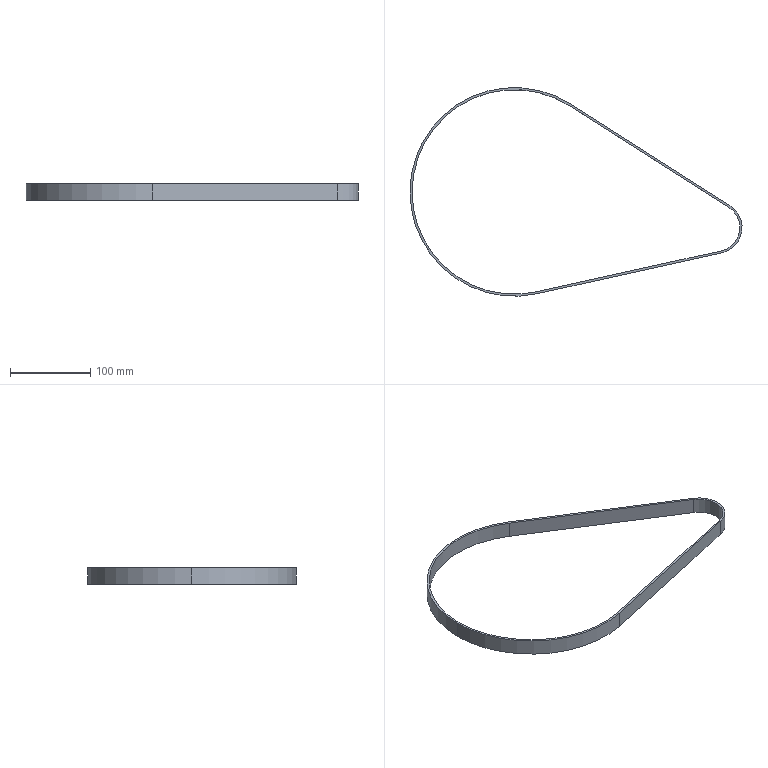Part | STEP file | Belt 1-8^ tube-changer assembly SGN-2 | 1 solid | 12 faces | box 413.576 x 259.89 x 20 mm | volume 55011 mm3 | cylinder 6 | plane 6 | commonest cylinder face diameters 254.65 x2 259.89 x2 59.74 x1 64.98 x1
STEP:
#1=CARTESIAN_POINT('',(0.,0.,0.));
#2=DIRECTION('',(0.,0.,1.));
#3=DIRECTION('',(1.,0.,0.));
#4=AXIS2_PLACEMENT_3D('',#1,#2,#3);
#5=CARTESIAN_POINT('',(-174.515,128.116,20.));
#6=VERTEX_POINT('',#5);
#7=CARTESIAN_POINT('',(-174.515,128.116,0.));
#8=VERTEX_POINT('',#7);
#9=CARTESIAN_POINT('',(-174.515,128.116,20.));
#10=DIRECTION('',(0.,0.,-1.));
#11=VECTOR('',#10,1.);
#12=LINE('',#9,#11);
#13=CARTESIAN_POINT('',(-242.865,20.692,20.));
#14=DIRECTION('',(0.,0.,-1.));
#15=DIRECTION('',(-1.,0.,0.));
#16=AXIS2_PLACEMENT_3D('',#13,#14,#15);
#17=CYLINDRICAL_SURFACE('',#16,127.325);
#18=CARTESIAN_POINT('',(2.137,0.));
#19=DIRECTION('',(0.,1.));
#20=VECTOR('',#19,1.);
#21=LINE('',#18,#20);
#22=(GEOMETRIC_REPRESENTATION_CONTEXT(2)PARAMETRIC_REPRESENTATION_CONTEXT()REPRESENTATION_CONTEXT('',''));
#23=DEFINITIONAL_REPRESENTATION('',(#21),#22);
#24=PCURVE('',#17,#23);
#25=CARTESIAN_POINT('',(-174.515,128.116,20.));
#26=DIRECTION('',(0.5368,0.8437,0.));
#27=DIRECTION('',(-0.8437,0.5368,0.));
#28=AXIS2_PLACEMENT_3D('',#25,#26,#27);
#29=PLANE('',#28);
#30=CARTESIAN_POINT('',(0.,0.));
#31=DIRECTION('',(0.,-1.));
#32=VECTOR('',#31,1.);
#33=LINE('',#30,#32);
#34=(GEOMETRIC_REPRESENTATION_CONTEXT(2)PARAMETRIC_REPRESENTATION_CONTEXT()REPRESENTATION_CONTEXT('',''));
#35=DEFINITIONAL_REPRESENTATION('',(#33),#34);
#36=PCURVE('',#29,#35);
#37=SURFACE_CURVE('',#12,(#24,#36),.PCURVE_S1.);
#38=EDGE_CURVE('',#6,#8,#37,.T.);
#39=ORIENTED_EDGE('',*,*,#38,.T.);
#40=CARTESIAN_POINT('',(-370.19,20.692,0.));
#41=VERTEX_POINT('',#40);
#42=CARTESIAN_POINT('',(-242.865,20.692,0.));
#43=DIRECTION('',(0.,0.,-1.));
#44=DIRECTION('',(-1.,0.,0.));
#45=AXIS2_PLACEMENT_3D('',#42,#43,#44);
#46=CIRCLE('',#45,127.325);
#47=CARTESIAN_POINT('',(0.,20.));
#48=DIRECTION('',(1.,0.));
#49=VECTOR('',#48,1.);
#50=LINE('',#47,#49);
#51=(GEOMETRIC_REPRESENTATION_CONTEXT(2)PARAMETRIC_REPRESENTATION_CONTEXT()REPRESENTATION_CONTEXT('',''));
#52=DEFINITIONAL_REPRESENTATION('',(#50),#51);
#53=PCURVE('',#17,#52);
#54=CARTESIAN_POINT('',(-242.865,20.692,0.));
#55=DIRECTION('',(0.,0.,-1.));
#56=DIRECTION('',(-1.,0.,0.));
#57=AXIS2_PLACEMENT_3D('',#54,#55,#56);
#58=PLANE('',#57);
#59=CARTESIAN_POINT('',(0.,0.));
#60=DIRECTION('',(1.,0.));
#61=AXIS2_PLACEMENT_2D('',#59,#60);
#62=CIRCLE('',#61,127.325);
#63=(GEOMETRIC_REPRESENTATION_CONTEXT(2)PARAMETRIC_REPRESENTATION_CONTEXT()REPRESENTATION_CONTEXT('',''));
#64=DEFINITIONAL_REPRESENTATION('',(#62),#63);
#65=PCURVE('',#58,#64);
#66=SURFACE_CURVE('',#46,(#53,#65),.PCURVE_S1.);
#67=EDGE_CURVE('',#41,#8,#66,.T.);
#68=ORIENTED_EDGE('',*,*,#67,.F.);
#69=CARTESIAN_POINT('',(-370.19,20.692,20.));
#70=VERTEX_POINT('',#69);
#71=CARTESIAN_POINT('',(-370.19,20.692,20.));
#72=DIRECTION('',(0.,0.,-1.));
#73=VECTOR('',#72,1.);
#74=LINE('',#71,#73);
#75=CARTESIAN_POINT('',(0.,0.));
#76=DIRECTION('',(0.,1.));
#77=VECTOR('',#76,1.);
#78=LINE('',#75,#77);
#79=(GEOMETRIC_REPRESENTATION_CONTEXT(2)PARAMETRIC_REPRESENTATION_CONTEXT()REPRESENTATION_CONTEXT('',''));
#80=DEFINITIONAL_REPRESENTATION('',(#78),#79);
#81=PCURVE('',#17,#80);
#82=CARTESIAN_POINT('',(-242.865,20.692,20.));
#83=DIRECTION('',(0.,0.,-1.));
#84=DIRECTION('',(-1.,0.,0.));
#85=AXIS2_PLACEMENT_3D('',#82,#83,#84);
#86=CYLINDRICAL_SURFACE('',#85,127.325);
#87=CARTESIAN_POINT('',(6.283,0.));
#88=DIRECTION('',(0.,1.));
#89=VECTOR('',#88,1.);
#90=LINE('',#87,#89);
#91=(GEOMETRIC_REPRESENTATION_CONTEXT(2)PARAMETRIC_REPRESENTATION_CONTEXT()REPRESENTATION_CONTEXT('',''));
#92=DEFINITIONAL_REPRESENTATION('',(#90),#91);
#93=PCURVE('',#86,#92);
#94=SURFACE_CURVE('',#74,(#81,#93),.PCURVE_S1.);
#95=EDGE_CURVE('',#70,#41,#94,.T.);
#96=ORIENTED_EDGE('',*,*,#95,.F.);
#97=CARTESIAN_POINT('',(-242.865,20.692,20.));
#98=DIRECTION('',(0.,0.,-1.));
#99=DIRECTION('',(-1.,0.,0.));
#100=AXIS2_PLACEMENT_3D('',#97,#98,#99);
#101=CIRCLE('',#100,127.325);
#102=CARTESIAN_POINT('',(0.,0.));
#103=DIRECTION('',(1.,0.));
#104=VECTOR('',#103,1.);
#105=LINE('',#102,#104);
#106=(GEOMETRIC_REPRESENTATION_CONTEXT(2)PARAMETRIC_REPRESENTATION_CONTEXT()REPRESENTATION_CONTEXT('',''));
#107=DEFINITIONAL_REPRESENTATION('',(#105),#106);
#108=PCURVE('',#17,#107);
#109=CARTESIAN_POINT('',(-242.865,20.692,20.));
#110=DIRECTION('',(0.,0.,-1.));
#111=DIRECTION('',(-1.,0.,0.));
#112=AXIS2_PLACEMENT_3D('',#109,#110,#111);
#113=PLANE('',#112);
#114=CARTESIAN_POINT('',(0.,0.));
#115=DIRECTION('',(1.,0.));
#116=AXIS2_PLACEMENT_2D('',#114,#115);
#117=CIRCLE('',#116,127.325);
#118=(GEOMETRIC_REPRESENTATION_CONTEXT(2)PARAMETRIC_REPRESENTATION_CONTEXT()REPRESENTATION_CONTEXT('',''));
#119=DEFINITIONAL_REPRESENTATION('',(#117),#118);
#120=PCURVE('',#113,#119);
#121=SURFACE_CURVE('',#101,(#108,#120),.PCURVE_S1.);
#122=EDGE_CURVE('',#70,#6,#121,.T.);
#123=ORIENTED_EDGE('',*,*,#122,.T.);
#124=EDGE_LOOP('',(#39,#68,#96,#123));
#125=FACE_BOUND('',#124,.F.);
#126=ADVANCED_FACE('',(#125),#17,.F.);
#127=CARTESIAN_POINT('',(-214.812,-106.188,20.));
#128=VERTEX_POINT('',#127);
#129=CARTESIAN_POINT('',(-372.81,20.692,20.));
#130=VERTEX_POINT('',#129);
#131=CARTESIAN_POINT('',(-242.865,20.692,20.));
#132=DIRECTION('',(0.,0.,-1.));
#133=DIRECTION('',(-1.,0.,0.));
#134=AXIS2_PLACEMENT_3D('',#131,#132,#133);
#135=CIRCLE('',#134,129.945);
#136=CARTESIAN_POINT('',(-242.865,20.692,20.));
#137=DIRECTION('',(0.,0.,-1.));
#138=DIRECTION('',(-1.,0.,0.));
#139=AXIS2_PLACEMENT_3D('',#136,#137,#138);
#140=CYLINDRICAL_SURFACE('',#139,129.945);
#141=CARTESIAN_POINT('',(0.,0.));
#142=DIRECTION('',(1.,0.));
#143=VECTOR('',#142,1.);
#144=LINE('',#141,#143);
#145=(GEOMETRIC_REPRESENTATION_CONTEXT(2)PARAMETRIC_REPRESENTATION_CONTEXT()REPRESENTATION_CONTEXT('',''));
#146=DEFINITIONAL_REPRESENTATION('',(#144),#145);
#147=PCURVE('',#140,#146);
#148=CARTESIAN_POINT('',(0.,0.));
#149=DIRECTION('',(1.,0.));
#150=AXIS2_PLACEMENT_2D('',#148,#149);
#151=CIRCLE('',#150,129.945);
#152=(GEOMETRIC_REPRESENTATION_CONTEXT(2)PARAMETRIC_REPRESENTATION_CONTEXT()REPRESENTATION_CONTEXT('',''));
#153=DEFINITIONAL_REPRESENTATION('',(#151),#152);
#154=PCURVE('',#113,#153);
#155=SURFACE_CURVE('',#135,(#147,#154),.PCURVE_S1.);
#156=EDGE_CURVE('',#128,#130,#155,.T.);
#157=ORIENTED_EDGE('',*,*,#156,.T.);
#158=CARTESIAN_POINT('',(-372.81,20.692,0.));
#159=VERTEX_POINT('',#158);
#160=CARTESIAN_POINT('',(-372.81,20.692,20.));
#161=DIRECTION('',(0.,0.,-1.));
#162=VECTOR('',#161,1.);
#163=LINE('',#160,#162);
#164=CARTESIAN_POINT('',(6.283,0.));
#165=DIRECTION('',(0.,1.));
#166=VECTOR('',#165,1.);
#167=LINE('',#164,#166);
#168=(GEOMETRIC_REPRESENTATION_CONTEXT(2)PARAMETRIC_REPRESENTATION_CONTEXT()REPRESENTATION_CONTEXT('',''));
#169=DEFINITIONAL_REPRESENTATION('',(#167),#168);
#170=PCURVE('',#140,#169);
#171=CARTESIAN_POINT('',(-242.865,20.692,20.));
#172=DIRECTION('',(0.,0.,-1.));
#173=DIRECTION('',(-1.,0.,0.));
#174=AXIS2_PLACEMENT_3D('',#171,#172,#173);
#175=CYLINDRICAL_SURFACE('',#174,129.945);
#176=CARTESIAN_POINT('',(0.,0.));
#177=DIRECTION('',(0.,1.));
#178=VECTOR('',#177,1.);
#179=LINE('',#176,#178);
#180=(GEOMETRIC_REPRESENTATION_CONTEXT(2)PARAMETRIC_REPRESENTATION_CONTEXT()REPRESENTATION_CONTEXT('',''));
#181=DEFINITIONAL_REPRESENTATION('',(#179),#180);
#182=PCURVE('',#175,#181);
#183=SURFACE_CURVE('',#163,(#170,#182),.PCURVE_S1.);
#184=EDGE_CURVE('',#130,#159,#183,.T.);
#185=ORIENTED_EDGE('',*,*,#184,.T.);
#186=CARTESIAN_POINT('',(-214.812,-106.188,0.));
#187=VERTEX_POINT('',#186);
#188=CARTESIAN_POINT('',(-242.865,20.692,0.));
#189=DIRECTION('',(0.,0.,-1.));
#190=DIRECTION('',(-1.,0.,0.));
#191=AXIS2_PLACEMENT_3D('',#188,#189,#190);
#192=CIRCLE('',#191,129.945);
#193=CARTESIAN_POINT('',(0.,20.));
#194=DIRECTION('',(1.,0.));
#195=VECTOR('',#194,1.);
#196=LINE('',#193,#195);
#197=(GEOMETRIC_REPRESENTATION_CONTEXT(2)PARAMETRIC_REPRESENTATION_CONTEXT()REPRESENTATION_CONTEXT('',''));
#198=DEFINITIONAL_REPRESENTATION('',(#196),#197);
#199=PCURVE('',#140,#198);
#200=CARTESIAN_POINT('',(0.,0.));
#201=DIRECTION('',(1.,0.));
#202=AXIS2_PLACEMENT_2D('',#200,#201);
#203=CIRCLE('',#202,129.945);
#204=(GEOMETRIC_REPRESENTATION_CONTEXT(2)PARAMETRIC_REPRESENTATION_CONTEXT()REPRESENTATION_CONTEXT('',''));
#205=DEFINITIONAL_REPRESENTATION('',(#203),#204);
#206=PCURVE('',#58,#205);
#207=SURFACE_CURVE('',#192,(#199,#206),.PCURVE_S1.);
#208=EDGE_CURVE('',#187,#159,#207,.T.);
#209=ORIENTED_EDGE('',*,*,#208,.F.);
#210=CARTESIAN_POINT('',(-214.812,-106.188,20.));
#211=DIRECTION('',(0.,0.,-1.));
#212=VECTOR('',#211,1.);
#213=LINE('',#210,#212);
#214=CARTESIAN_POINT('',(4.495,0.));
#215=DIRECTION('',(0.,1.));
#216=VECTOR('',#215,1.);
#217=LINE('',#214,#216);
#218=(GEOMETRIC_REPRESENTATION_CONTEXT(2)PARAMETRIC_REPRESENTATION_CONTEXT()REPRESENTATION_CONTEXT('',''));
#219=DEFINITIONAL_REPRESENTATION('',(#217),#218);
#220=PCURVE('',#140,#219);
#221=CARTESIAN_POINT('',(-214.812,-106.188,20.));
#222=DIRECTION('',(0.2159,-0.9764,0.));
#223=DIRECTION('',(0.9764,0.2159,0.));
#224=AXIS2_PLACEMENT_3D('',#221,#222,#223);
#225=PLANE('',#224);
#226=CARTESIAN_POINT('',(0.,0.));
#227=DIRECTION('',(0.,-1.));
#228=VECTOR('',#227,1.);
#229=LINE('',#226,#228);
#230=(GEOMETRIC_REPRESENTATION_CONTEXT(2)PARAMETRIC_REPRESENTATION_CONTEXT()REPRESENTATION_CONTEXT('',''));
#231=DEFINITIONAL_REPRESENTATION('',(#229),#230);
#232=PCURVE('',#225,#231);
#233=SURFACE_CURVE('',#213,(#220,#232),.PCURVE_S1.);
#234=EDGE_CURVE('',#128,#187,#233,.T.);
#235=ORIENTED_EDGE('',*,*,#234,.F.);
#236=EDGE_LOOP('',(#157,#185,#209,#235));
#237=FACE_BOUND('',#236,.T.);
#238=ADVANCED_FACE('',(#237),#140,.T.);
#239=ORIENTED_EDGE('',*,*,#184,.F.);
#240=CARTESIAN_POINT('',(-173.108,130.327,20.));
#241=VERTEX_POINT('',#240);
#242=CARTESIAN_POINT('',(-242.865,20.692,20.));
#243=DIRECTION('',(0.,0.,-1.));
#244=DIRECTION('',(-1.,0.,0.));
#245=AXIS2_PLACEMENT_3D('',#242,#243,#244);
#246=CIRCLE('',#245,129.945);
#247=CARTESIAN_POINT('',(0.,0.));
#248=DIRECTION('',(1.,0.));
#249=VECTOR('',#248,1.);
#250=LINE('',#247,#249);
#251=(GEOMETRIC_REPRESENTATION_CONTEXT(2)PARAMETRIC_REPRESENTATION_CONTEXT()REPRESENTATION_CONTEXT('',''));
#252=DEFINITIONAL_REPRESENTATION('',(#250),#251);
#253=PCURVE('',#175,#252);
#254=CARTESIAN_POINT('',(0.,0.));
#255=DIRECTION('',(1.,0.));
#256=AXIS2_PLACEMENT_2D('',#254,#255);
#257=CIRCLE('',#256,129.945);
#258=(GEOMETRIC_REPRESENTATION_CONTEXT(2)PARAMETRIC_REPRESENTATION_CONTEXT()REPRESENTATION_CONTEXT('',''));
#259=DEFINITIONAL_REPRESENTATION('',(#257),#258);
#260=PCURVE('',#113,#259);
#261=SURFACE_CURVE('',#246,(#253,#260),.PCURVE_S1.);
#262=EDGE_CURVE('',#130,#241,#261,.T.);
#263=ORIENTED_EDGE('',*,*,#262,.T.);
#264=CARTESIAN_POINT('',(-173.108,130.327,0.));
#265=VERTEX_POINT('',#264);
#266=CARTESIAN_POINT('',(-173.108,130.327,20.));
#267=DIRECTION('',(0.,0.,-1.));
#268=VECTOR('',#267,1.);
#269=LINE('',#266,#268);
#270=CARTESIAN_POINT('',(2.137,0.));
#271=DIRECTION('',(0.,1.));
#272=VECTOR('',#271,1.);
#273=LINE('',#270,#272);
#274=(GEOMETRIC_REPRESENTATION_CONTEXT(2)PARAMETRIC_REPRESENTATION_CONTEXT()REPRESENTATION_CONTEXT('',''));
#275=DEFINITIONAL_REPRESENTATION('',(#273),#274);
#276=PCURVE('',#175,#275);
#277=CARTESIAN_POINT('',(-173.108,130.327,20.));
#278=DIRECTION('',(0.5368,0.8437,0.));
#279=DIRECTION('',(-0.8437,0.5368,0.));
#280=AXIS2_PLACEMENT_3D('',#277,#278,#279);
#281=PLANE('',#280);
#282=CARTESIAN_POINT('',(0.,0.));
#283=DIRECTION('',(0.,-1.));
#284=VECTOR('',#283,1.);
#285=LINE('',#282,#284);
#286=(GEOMETRIC_REPRESENTATION_CONTEXT(2)PARAMETRIC_REPRESENTATION_CONTEXT()REPRESENTATION_CONTEXT('',''));
#287=DEFINITIONAL_REPRESENTATION('',(#285),#286);
#288=PCURVE('',#281,#287);
#289=SURFACE_CURVE('',#269,(#276,#288),.PCURVE_S1.);
#290=EDGE_CURVE('',#241,#265,#289,.T.);
#291=ORIENTED_EDGE('',*,*,#290,.T.);
#292=CARTESIAN_POINT('',(-242.865,20.692,0.));
#293=DIRECTION('',(0.,0.,-1.));
#294=DIRECTION('',(-1.,0.,0.));
#295=AXIS2_PLACEMENT_3D('',#292,#293,#294);
#296=CIRCLE('',#295,129.945);
#297=CARTESIAN_POINT('',(0.,20.));
#298=DIRECTION('',(1.,0.));
#299=VECTOR('',#298,1.);
#300=LINE('',#297,#299);
#301=(GEOMETRIC_REPRESENTATION_CONTEXT(2)PARAMETRIC_REPRESENTATION_CONTEXT()REPRESENTATION_CONTEXT('',''));
#302=DEFINITIONAL_REPRESENTATION('',(#300),#301);
#303=PCURVE('',#175,#302);
#304=CARTESIAN_POINT('',(0.,0.));
#305=DIRECTION('',(1.,0.));
#306=AXIS2_PLACEMENT_2D('',#304,#305);
#307=CIRCLE('',#306,129.945);
#308=(GEOMETRIC_REPRESENTATION_CONTEXT(2)PARAMETRIC_REPRESENTATION_CONTEXT()REPRESENTATION_CONTEXT('',''));
#309=DEFINITIONAL_REPRESENTATION('',(#307),#308);
#310=PCURVE('',#58,#309);
#311=SURFACE_CURVE('',#296,(#303,#310),.PCURVE_S1.);
#312=EDGE_CURVE('',#159,#265,#311,.T.);
#313=ORIENTED_EDGE('',*,*,#312,.F.);
#314=EDGE_LOOP('',(#239,#263,#291,#313));
#315=FACE_BOUND('',#314,.T.);
#316=ADVANCED_FACE('',(#315),#175,.T.);
#317=CARTESIAN_POINT('',(15.29,-55.314,0.));
#318=VERTEX_POINT('',#317);
#319=CARTESIAN_POINT('',(-214.812,-106.188,0.));
#320=DIRECTION('',(-0.9764,-0.2159,0.));
#321=VECTOR('',#320,1.);
#322=LINE('',#319,#321);
#323=CARTESIAN_POINT('',(0.,-20.));
#324=DIRECTION('',(-1.,0.));
#325=VECTOR('',#324,1.);
#326=LINE('',#323,#325);
#327=(GEOMETRIC_REPRESENTATION_CONTEXT(2)PARAMETRIC_REPRESENTATION_CONTEXT()REPRESENTATION_CONTEXT('',''));
#328=DEFINITIONAL_REPRESENTATION('',(#326),#327);
#329=PCURVE('',#225,#328);
#330=CARTESIAN_POINT('',(-28.053,-126.881));
#331=DIRECTION('',(0.9764,-0.2159));
#332=VECTOR('',#331,1.);
#333=LINE('',#330,#332);
#334=(GEOMETRIC_REPRESENTATION_CONTEXT(2)PARAMETRIC_REPRESENTATION_CONTEXT()REPRESENTATION_CONTEXT('',''));
#335=DEFINITIONAL_REPRESENTATION('',(#333),#334);
#336=PCURVE('',#58,#335);
#337=SURFACE_CURVE('',#322,(#329,#336),.PCURVE_S1.);
#338=EDGE_CURVE('',#318,#187,#337,.T.);
#339=ORIENTED_EDGE('',*,*,#338,.F.);
#340=CARTESIAN_POINT('',(15.29,-55.314,20.));
#341=VERTEX_POINT('',#340);
#342=CARTESIAN_POINT('',(15.29,-55.314,20.));
#343=DIRECTION('',(0.,0.,-1.));
#344=VECTOR('',#343,1.);
#345=LINE('',#342,#344);
#346=CARTESIAN_POINT('',(235.659,0.));
#347=DIRECTION('',(0.,-1.));
#348=VECTOR('',#347,1.);
#349=LINE('',#346,#348);
#350=(GEOMETRIC_REPRESENTATION_CONTEXT(2)PARAMETRIC_REPRESENTATION_CONTEXT()REPRESENTATION_CONTEXT('',''));
#351=DEFINITIONAL_REPRESENTATION('',(#349),#350);
#352=PCURVE('',#225,#351);
#353=CARTESIAN_POINT('',(8.276,-23.59,20.));
#354=DIRECTION('',(0.,0.,-1.));
#355=DIRECTION('',(-1.,0.,0.));
#356=AXIS2_PLACEMENT_3D('',#353,#354,#355);
#357=CYLINDRICAL_SURFACE('',#356,32.49);
#358=CARTESIAN_POINT('',(4.495,0.));
#359=DIRECTION('',(0.,1.));
#360=VECTOR('',#359,1.);
#361=LINE('',#358,#360);
#362=(GEOMETRIC_REPRESENTATION_CONTEXT(2)PARAMETRIC_REPRESENTATION_CONTEXT()REPRESENTATION_CONTEXT('',''));
#363=DEFINITIONAL_REPRESENTATION('',(#361),#362);
#364=PCURVE('',#357,#363);
#365=SURFACE_CURVE('',#345,(#352,#364),.PCURVE_S1.);
#366=EDGE_CURVE('',#341,#318,#365,.T.);
#367=ORIENTED_EDGE('',*,*,#366,.F.);
#368=CARTESIAN_POINT('',(-214.812,-106.188,20.));
#369=DIRECTION('',(-0.9764,-0.2159,0.));
#370=VECTOR('',#369,1.);
#371=LINE('',#368,#370);
#372=CARTESIAN_POINT('',(0.,0.));
#373=DIRECTION('',(-1.,0.));
#374=VECTOR('',#373,1.);
#375=LINE('',#372,#374);
#376=(GEOMETRIC_REPRESENTATION_CONTEXT(2)PARAMETRIC_REPRESENTATION_CONTEXT()REPRESENTATION_CONTEXT('',''));
#377=DEFINITIONAL_REPRESENTATION('',(#375),#376);
#378=PCURVE('',#225,#377);
#379=CARTESIAN_POINT('',(-28.053,-126.881));
#380=DIRECTION('',(0.9764,-0.2159));
#381=VECTOR('',#380,1.);
#382=LINE('',#379,#381);
#383=(GEOMETRIC_REPRESENTATION_CONTEXT(2)PARAMETRIC_REPRESENTATION_CONTEXT()REPRESENTATION_CONTEXT('',''));
#384=DEFINITIONAL_REPRESENTATION('',(#382),#383);
#385=PCURVE('',#113,#384);
#386=SURFACE_CURVE('',#371,(#378,#385),.PCURVE_S1.);
#387=EDGE_CURVE('',#341,#128,#386,.T.);
#388=ORIENTED_EDGE('',*,*,#387,.T.);
#389=ORIENTED_EDGE('',*,*,#234,.T.);
#390=EDGE_LOOP('',(#339,#367,#388,#389));
#391=FACE_BOUND('',#390,.T.);
#392=ADVANCED_FACE('',(#391),#225,.T.);
#393=CARTESIAN_POINT('',(25.717,3.821,0.));
#394=VERTEX_POINT('',#393);
#395=CARTESIAN_POINT('',(8.276,-23.59,0.));
#396=DIRECTION('',(0.,0.,-1.));
#397=DIRECTION('',(-1.,0.,0.));
#398=AXIS2_PLACEMENT_3D('',#395,#396,#397);
#399=CIRCLE('',#398,32.49);
#400=CARTESIAN_POINT('',(0.,20.));
#401=DIRECTION('',(1.,0.));
#402=VECTOR('',#401,1.);
#403=LINE('',#400,#402);
#404=(GEOMETRIC_REPRESENTATION_CONTEXT(2)PARAMETRIC_REPRESENTATION_CONTEXT()REPRESENTATION_CONTEXT('',''));
#405=DEFINITIONAL_REPRESENTATION('',(#403),#404);
#406=PCURVE('',#357,#405);
#407=CARTESIAN_POINT('',(-251.141,-44.283));
#408=DIRECTION('',(1.,0.));
#409=AXIS2_PLACEMENT_2D('',#407,#408);
#410=CIRCLE('',#409,32.49);
#411=(GEOMETRIC_REPRESENTATION_CONTEXT(2)PARAMETRIC_REPRESENTATION_CONTEXT()REPRESENTATION_CONTEXT('',''));
#412=DEFINITIONAL_REPRESENTATION('',(#410),#411);
#413=PCURVE('',#58,#412);
#414=SURFACE_CURVE('',#399,(#406,#413),.PCURVE_S1.);
#415=EDGE_CURVE('',#394,#318,#414,.T.);
#416=ORIENTED_EDGE('',*,*,#415,.F.);
#417=CARTESIAN_POINT('',(25.717,3.821,20.));
#418=VERTEX_POINT('',#417);
#419=CARTESIAN_POINT('',(25.717,3.821,20.));
#420=DIRECTION('',(0.,0.,-1.));
#421=VECTOR('',#420,1.);
#422=LINE('',#419,#421);
#423=CARTESIAN_POINT('',(2.137,0.));
#424=DIRECTION('',(0.,1.));
#425=VECTOR('',#424,1.);
#426=LINE('',#423,#425);
#427=(GEOMETRIC_REPRESENTATION_CONTEXT(2)PARAMETRIC_REPRESENTATION_CONTEXT()REPRESENTATION_CONTEXT('',''));
#428=DEFINITIONAL_REPRESENTATION('',(#426),#427);
#429=PCURVE('',#357,#428);
#430=CARTESIAN_POINT('',(-235.659,0.));
#431=DIRECTION('',(0.,-1.));
#432=VECTOR('',#431,1.);
#433=LINE('',#430,#432);
#434=(GEOMETRIC_REPRESENTATION_CONTEXT(2)PARAMETRIC_REPRESENTATION_CONTEXT()REPRESENTATION_CONTEXT('',''));
#435=DEFINITIONAL_REPRESENTATION('',(#433),#434);
#436=PCURVE('',#281,#435);
#437=SURFACE_CURVE('',#422,(#429,#436),.PCURVE_S1.);
#438=EDGE_CURVE('',#418,#394,#437,.T.);
#439=ORIENTED_EDGE('',*,*,#438,.F.);
#440=CARTESIAN_POINT('',(8.276,-23.59,20.));
#441=DIRECTION('',(0.,0.,-1.));
#442=DIRECTION('',(-1.,0.,0.));
#443=AXIS2_PLACEMENT_3D('',#440,#441,#442);
#444=CIRCLE('',#443,32.49);
#445=CARTESIAN_POINT('',(0.,0.));
#446=DIRECTION('',(1.,0.));
#447=VECTOR('',#446,1.);
#448=LINE('',#445,#447);
#449=(GEOMETRIC_REPRESENTATION_CONTEXT(2)PARAMETRIC_REPRESENTATION_CONTEXT()REPRESENTATION_CONTEXT('',''));
#450=DEFINITIONAL_REPRESENTATION('',(#448),#449);
#451=PCURVE('',#357,#450);
#452=CARTESIAN_POINT('',(-251.141,-44.283));
#453=DIRECTION('',(1.,0.));
#454=AXIS2_PLACEMENT_2D('',#452,#453);
#455=CIRCLE('',#454,32.49);
#456=(GEOMETRIC_REPRESENTATION_CONTEXT(2)PARAMETRIC_REPRESENTATION_CONTEXT()REPRESENTATION_CONTEXT('',''));
#457=DEFINITIONAL_REPRESENTATION('',(#455),#456);
#458=PCURVE('',#113,#457);
#459=SURFACE_CURVE('',#444,(#451,#458),.PCURVE_S1.);
#460=EDGE_CURVE('',#418,#341,#459,.T.);
#461=ORIENTED_EDGE('',*,*,#460,.T.);
#462=ORIENTED_EDGE('',*,*,#366,.T.);
#463=EDGE_LOOP('',(#416,#439,#461,#462));
#464=FACE_BOUND('',#463,.T.);
#465=ADVANCED_FACE('',(#464),#357,.T.);
#466=CARTESIAN_POINT('',(-173.108,130.327,0.));
#467=DIRECTION('',(0.8437,-0.5368,0.));
#468=VECTOR('',#467,1.);
#469=LINE('',#466,#468);
#470=CARTESIAN_POINT('',(0.,-20.));
#471=DIRECTION('',(-1.,0.));
#472=VECTOR('',#471,1.);
#473=LINE('',#470,#472);
#474=(GEOMETRIC_REPRESENTATION_CONTEXT(2)PARAMETRIC_REPRESENTATION_CONTEXT()REPRESENTATION_CONTEXT('',''));
#475=DEFINITIONAL_REPRESENTATION('',(#473),#474);
#476=PCURVE('',#281,#475);
#477=CARTESIAN_POINT('',(-69.757,109.634));
#478=DIRECTION('',(-0.8437,-0.5368));
#479=VECTOR('',#478,1.);
#480=LINE('',#477,#479);
#481=(GEOMETRIC_REPRESENTATION_CONTEXT(2)PARAMETRIC_REPRESENTATION_CONTEXT()REPRESENTATION_CONTEXT('',''));
#482=DEFINITIONAL_REPRESENTATION('',(#480),#481);
#483=PCURVE('',#58,#482);
#484=SURFACE_CURVE('',#469,(#476,#483),.PCURVE_S1.);
#485=EDGE_CURVE('',#265,#394,#484,.T.);
#486=ORIENTED_EDGE('',*,*,#485,.F.);
#487=ORIENTED_EDGE('',*,*,#290,.F.);
#488=CARTESIAN_POINT('',(-173.108,130.327,20.));
#489=DIRECTION('',(0.8437,-0.5368,0.));
#490=VECTOR('',#489,1.);
#491=LINE('',#488,#490);
#492=CARTESIAN_POINT('',(0.,0.));
#493=DIRECTION('',(-1.,0.));
#494=VECTOR('',#493,1.);
#495=LINE('',#492,#494);
#496=(GEOMETRIC_REPRESENTATION_CONTEXT(2)PARAMETRIC_REPRESENTATION_CONTEXT()REPRESENTATION_CONTEXT('',''));
#497=DEFINITIONAL_REPRESENTATION('',(#495),#496);
#498=PCURVE('',#281,#497);
#499=CARTESIAN_POINT('',(-69.757,109.634));
#500=DIRECTION('',(-0.8437,-0.5368));
#501=VECTOR('',#500,1.);
#502=LINE('',#499,#501);
#503=(GEOMETRIC_REPRESENTATION_CONTEXT(2)PARAMETRIC_REPRESENTATION_CONTEXT()REPRESENTATION_CONTEXT('',''));
#504=DEFINITIONAL_REPRESENTATION('',(#502),#503);
#505=PCURVE('',#113,#504);
#506=SURFACE_CURVE('',#491,(#498,#505),.PCURVE_S1.);
#507=EDGE_CURVE('',#241,#418,#506,.T.);
#508=ORIENTED_EDGE('',*,*,#507,.T.);
#509=ORIENTED_EDGE('',*,*,#438,.T.);
#510=EDGE_LOOP('',(#486,#487,#508,#509));
#511=FACE_BOUND('',#510,.T.);
#512=ADVANCED_FACE('',(#511),#281,.T.);
#513=CARTESIAN_POINT('',(14.724,-52.756,20.));
#514=VERTEX_POINT('',#513);
#515=CARTESIAN_POINT('',(-215.378,-103.63,20.));
#516=VERTEX_POINT('',#515);
#517=CARTESIAN_POINT('',(14.724,-52.756,20.));
#518=DIRECTION('',(-0.9764,-0.2159,0.));
#519=VECTOR('',#518,1.);
#520=LINE('',#517,#519);
#521=CARTESIAN_POINT('',(-257.589,-73.449));
#522=DIRECTION('',(0.9764,-0.2159));
#523=VECTOR('',#522,1.);
#524=LINE('',#521,#523);
#525=(GEOMETRIC_REPRESENTATION_CONTEXT(2)PARAMETRIC_REPRESENTATION_CONTEXT()REPRESENTATION_CONTEXT('',''));
#526=DEFINITIONAL_REPRESENTATION('',(#524),#525);
#527=PCURVE('',#113,#526);
#528=CARTESIAN_POINT('',(14.724,-52.756,20.));
#529=DIRECTION('',(0.2159,-0.9764,0.));
#530=DIRECTION('',(0.9764,0.2159,0.));
#531=AXIS2_PLACEMENT_3D('',#528,#529,#530);
#532=PLANE('',#531);
#533=CARTESIAN_POINT('',(0.,0.));
#534=DIRECTION('',(-1.,0.));
#535=VECTOR('',#534,1.);
#536=LINE('',#533,#535);
#537=(GEOMETRIC_REPRESENTATION_CONTEXT(2)PARAMETRIC_REPRESENTATION_CONTEXT()REPRESENTATION_CONTEXT('',''));
#538=DEFINITIONAL_REPRESENTATION('',(#536),#537);
#539=PCURVE('',#532,#538);
#540=SURFACE_CURVE('',#520,(#527,#539),.PCURVE_S1.);
#541=EDGE_CURVE('',#514,#516,#540,.T.);
#542=ORIENTED_EDGE('',*,*,#541,.T.);
#543=CARTESIAN_POINT('',(-242.865,20.692,20.));
#544=DIRECTION('',(0.,0.,-1.));
#545=DIRECTION('',(-1.,0.,0.));
#546=AXIS2_PLACEMENT_3D('',#543,#544,#545);
#547=CIRCLE('',#546,127.325);
#548=CARTESIAN_POINT('',(0.,0.));
#549=DIRECTION('',(1.,0.));
#550=AXIS2_PLACEMENT_2D('',#548,#549);
#551=CIRCLE('',#550,127.325);
#552=(GEOMETRIC_REPRESENTATION_CONTEXT(2)PARAMETRIC_REPRESENTATION_CONTEXT()REPRESENTATION_CONTEXT('',''));
#553=DEFINITIONAL_REPRESENTATION('',(#551),#552);
#554=PCURVE('',#113,#553);
#555=CARTESIAN_POINT('',(0.,0.));
#556=DIRECTION('',(1.,0.));
#557=VECTOR('',#556,1.);
#558=LINE('',#555,#557);
#559=(GEOMETRIC_REPRESENTATION_CONTEXT(2)PARAMETRIC_REPRESENTATION_CONTEXT()REPRESENTATION_CONTEXT('',''));
#560=DEFINITIONAL_REPRESENTATION('',(#558),#559);
#561=PCURVE('',#86,#560);
#562=SURFACE_CURVE('',#547,(#554,#561),.PCURVE_S1.);
#563=EDGE_CURVE('',#516,#70,#562,.T.);
#564=ORIENTED_EDGE('',*,*,#563,.T.);
#565=ORIENTED_EDGE('',*,*,#122,.T.);
#566=CARTESIAN_POINT('',(24.311,1.611,20.));
#567=VERTEX_POINT('',#566);
#568=CARTESIAN_POINT('',(-174.515,128.116,20.));
#569=DIRECTION('',(0.8437,-0.5368,0.));
#570=VECTOR('',#569,1.);
#571=LINE('',#568,#570);
#572=CARTESIAN_POINT('',(-68.35,107.424));
#573=DIRECTION('',(-0.8437,-0.5368));
#574=VECTOR('',#573,1.);
#575=LINE('',#572,#574);
#576=(GEOMETRIC_REPRESENTATION_CONTEXT(2)PARAMETRIC_REPRESENTATION_CONTEXT()REPRESENTATION_CONTEXT('',''));
#577=DEFINITIONAL_REPRESENTATION('',(#575),#576);
#578=PCURVE('',#113,#577);
#579=CARTESIAN_POINT('',(0.,0.));
#580=DIRECTION('',(-1.,0.));
#581=VECTOR('',#580,1.);
#582=LINE('',#579,#581);
#583=(GEOMETRIC_REPRESENTATION_CONTEXT(2)PARAMETRIC_REPRESENTATION_CONTEXT()REPRESENTATION_CONTEXT('',''));
#584=DEFINITIONAL_REPRESENTATION('',(#582),#583);
#585=PCURVE('',#29,#584);
#586=SURFACE_CURVE('',#571,(#578,#585),.PCURVE_S1.);
#587=EDGE_CURVE('',#6,#567,#586,.T.);
#588=ORIENTED_EDGE('',*,*,#587,.T.);
#589=CARTESIAN_POINT('',(8.276,-23.59,20.));
#590=DIRECTION('',(0.,0.,-1.));
#591=DIRECTION('',(-1.,0.,0.));
#592=AXIS2_PLACEMENT_3D('',#589,#590,#591);
#593=CIRCLE('',#592,29.87);
#594=CARTESIAN_POINT('',(-251.141,-44.283));
#595=DIRECTION('',(1.,0.));
#596=AXIS2_PLACEMENT_2D('',#594,#595);
#597=CIRCLE('',#596,29.87);
#598=(GEOMETRIC_REPRESENTATION_CONTEXT(2)PARAMETRIC_REPRESENTATION_CONTEXT()REPRESENTATION_CONTEXT('',''));
#599=DEFINITIONAL_REPRESENTATION('',(#597),#598);
#600=PCURVE('',#113,#599);
#601=CARTESIAN_POINT('',(8.276,-23.59,20.));
#602=DIRECTION('',(0.,0.,-1.));
#603=DIRECTION('',(-1.,0.,0.));
#604=AXIS2_PLACEMENT_3D('',#601,#602,#603);
#605=CYLINDRICAL_SURFACE('',#604,29.87);
#606=CARTESIAN_POINT('',(0.,0.));
#607=DIRECTION('',(1.,0.));
#608=VECTOR('',#607,1.);
#609=LINE('',#606,#608);
#610=(GEOMETRIC_REPRESENTATION_CONTEXT(2)PARAMETRIC_REPRESENTATION_CONTEXT()REPRESENTATION_CONTEXT('',''));
#611=DEFINITIONAL_REPRESENTATION('',(#609),#610);
#612=PCURVE('',#605,#611);
#613=SURFACE_CURVE('',#593,(#600,#612),.PCURVE_S1.);
#614=EDGE_CURVE('',#567,#514,#613,.T.);
#615=ORIENTED_EDGE('',*,*,#614,.T.);
#616=EDGE_LOOP('',(#542,#564,#565,#588,#615));
#617=FACE_BOUND('',#616,.T.);
#618=ORIENTED_EDGE('',*,*,#156,.F.);
#619=ORIENTED_EDGE('',*,*,#387,.F.);
#620=ORIENTED_EDGE('',*,*,#460,.F.);
#621=ORIENTED_EDGE('',*,*,#507,.F.);
#622=ORIENTED_EDGE('',*,*,#262,.F.);
#623=EDGE_LOOP('',(#618,#619,#620,#621,#622));
#624=FACE_BOUND('',#623,.T.);
#625=ADVANCED_FACE('',(#617,#624),#113,.F.);
#626=CARTESIAN_POINT('',(-215.378,-103.63,0.));
#627=VERTEX_POINT('',#626);
#628=CARTESIAN_POINT('',(-242.865,20.692,0.));
#629=DIRECTION('',(0.,0.,-1.));
#630=DIRECTION('',(-1.,0.,0.));
#631=AXIS2_PLACEMENT_3D('',#628,#629,#630);
#632=CIRCLE('',#631,127.325);
#633=CARTESIAN_POINT('',(0.,0.));
#634=DIRECTION('',(1.,0.));
#635=AXIS2_PLACEMENT_2D('',#633,#634);
#636=CIRCLE('',#635,127.325);
#637=(GEOMETRIC_REPRESENTATION_CONTEXT(2)PARAMETRIC_REPRESENTATION_CONTEXT()REPRESENTATION_CONTEXT('',''));
#638=DEFINITIONAL_REPRESENTATION('',(#636),#637);
#639=PCURVE('',#58,#638);
#640=CARTESIAN_POINT('',(0.,20.));
#641=DIRECTION('',(1.,0.));
#642=VECTOR('',#641,1.);
#643=LINE('',#640,#642);
#644=(GEOMETRIC_REPRESENTATION_CONTEXT(2)PARAMETRIC_REPRESENTATION_CONTEXT()REPRESENTATION_CONTEXT('',''));
#645=DEFINITIONAL_REPRESENTATION('',(#643),#644);
#646=PCURVE('',#86,#645);
#647=SURFACE_CURVE('',#632,(#639,#646),.PCURVE_S1.);
#648=EDGE_CURVE('',#627,#41,#647,.T.);
#649=ORIENTED_EDGE('',*,*,#648,.F.);
#650=CARTESIAN_POINT('',(14.724,-52.756,0.));
#651=VERTEX_POINT('',#650);
#652=CARTESIAN_POINT('',(14.724,-52.756,0.));
#653=DIRECTION('',(-0.9764,-0.2159,0.));
#654=VECTOR('',#653,1.);
#655=LINE('',#652,#654);
#656=CARTESIAN_POINT('',(-257.589,-73.449));
#657=DIRECTION('',(0.9764,-0.2159));
#658=VECTOR('',#657,1.);
#659=LINE('',#656,#658);
#660=(GEOMETRIC_REPRESENTATION_CONTEXT(2)PARAMETRIC_REPRESENTATION_CONTEXT()REPRESENTATION_CONTEXT('',''));
#661=DEFINITIONAL_REPRESENTATION('',(#659),#660);
#662=PCURVE('',#58,#661);
#663=CARTESIAN_POINT('',(0.,-20.));
#664=DIRECTION('',(-1.,0.));
#665=VECTOR('',#664,1.);
#666=LINE('',#663,#665);
#667=(GEOMETRIC_REPRESENTATION_CONTEXT(2)PARAMETRIC_REPRESENTATION_CONTEXT()REPRESENTATION_CONTEXT('',''));
#668=DEFINITIONAL_REPRESENTATION('',(#666),#667);
#669=PCURVE('',#532,#668);
#670=SURFACE_CURVE('',#655,(#662,#669),.PCURVE_S1.);
#671=EDGE_CURVE('',#651,#627,#670,.T.);
#672=ORIENTED_EDGE('',*,*,#671,.F.);
#673=CARTESIAN_POINT('',(24.311,1.611,0.));
#674=VERTEX_POINT('',#673);
#675=CARTESIAN_POINT('',(8.276,-23.59,0.));
#676=DIRECTION('',(0.,0.,-1.));
#677=DIRECTION('',(-1.,0.,0.));
#678=AXIS2_PLACEMENT_3D('',#675,#676,#677);
#679=CIRCLE('',#678,29.87);
#680=CARTESIAN_POINT('',(-251.141,-44.283));
#681=DIRECTION('',(1.,0.));
#682=AXIS2_PLACEMENT_2D('',#680,#681);
#683=CIRCLE('',#682,29.87);
#684=(GEOMETRIC_REPRESENTATION_CONTEXT(2)PARAMETRIC_REPRESENTATION_CONTEXT()REPRESENTATION_CONTEXT('',''));
#685=DEFINITIONAL_REPRESENTATION('',(#683),#684);
#686=PCURVE('',#58,#685);
#687=CARTESIAN_POINT('',(0.,20.));
#688=DIRECTION('',(1.,0.));
#689=VECTOR('',#688,1.);
#690=LINE('',#687,#689);
#691=(GEOMETRIC_REPRESENTATION_CONTEXT(2)PARAMETRIC_REPRESENTATION_CONTEXT()REPRESENTATION_CONTEXT('',''));
#692=DEFINITIONAL_REPRESENTATION('',(#690),#691);
#693=PCURVE('',#605,#692);
#694=SURFACE_CURVE('',#679,(#686,#693),.PCURVE_S1.);
#695=EDGE_CURVE('',#674,#651,#694,.T.);
#696=ORIENTED_EDGE('',*,*,#695,.F.);
#697=CARTESIAN_POINT('',(-174.515,128.116,0.));
#698=DIRECTION('',(0.8437,-0.5368,0.));
#699=VECTOR('',#698,1.);
#700=LINE('',#697,#699);
#701=CARTESIAN_POINT('',(-68.35,107.424));
#702=DIRECTION('',(-0.8437,-0.5368));
#703=VECTOR('',#702,1.);
#704=LINE('',#701,#703);
#705=(GEOMETRIC_REPRESENTATION_CONTEXT(2)PARAMETRIC_REPRESENTATION_CONTEXT()REPRESENTATION_CONTEXT('',''));
#706=DEFINITIONAL_REPRESENTATION('',(#704),#705);
#707=PCURVE('',#58,#706);
#708=CARTESIAN_POINT('',(0.,-20.));
#709=DIRECTION('',(-1.,0.));
#710=VECTOR('',#709,1.);
#711=LINE('',#708,#710);
#712=(GEOMETRIC_REPRESENTATION_CONTEXT(2)PARAMETRIC_REPRESENTATION_CONTEXT()REPRESENTATION_CONTEXT('',''));
#713=DEFINITIONAL_REPRESENTATION('',(#711),#712);
#714=PCURVE('',#29,#713);
#715=SURFACE_CURVE('',#700,(#707,#714),.PCURVE_S1.);
#716=EDGE_CURVE('',#8,#674,#715,.T.);
#717=ORIENTED_EDGE('',*,*,#716,.F.);
#718=ORIENTED_EDGE('',*,*,#67,.F.);
#719=EDGE_LOOP('',(#649,#672,#696,#717,#718));
#720=FACE_BOUND('',#719,.T.);
#721=ORIENTED_EDGE('',*,*,#208,.T.);
#722=ORIENTED_EDGE('',*,*,#312,.T.);
#723=ORIENTED_EDGE('',*,*,#485,.T.);
#724=ORIENTED_EDGE('',*,*,#415,.T.);
#725=ORIENTED_EDGE('',*,*,#338,.T.);
#726=EDGE_LOOP('',(#721,#722,#723,#724,#725));
#727=FACE_BOUND('',#726,.T.);
#728=ADVANCED_FACE('',(#720,#727),#58,.T.);
#729=ORIENTED_EDGE('',*,*,#648,.F.);
#730=CARTESIAN_POINT('',(-215.378,-103.63,20.));
#731=DIRECTION('',(0.,0.,-1.));
#732=VECTOR('',#731,1.);
#733=LINE('',#730,#732);
#734=CARTESIAN_POINT('',(4.495,0.));
#735=DIRECTION('',(0.,1.));
#736=VECTOR('',#735,1.);
#737=LINE('',#734,#736);
#738=(GEOMETRIC_REPRESENTATION_CONTEXT(2)PARAMETRIC_REPRESENTATION_CONTEXT()REPRESENTATION_CONTEXT('',''));
#739=DEFINITIONAL_REPRESENTATION('',(#737),#738);
#740=PCURVE('',#86,#739);
#741=CARTESIAN_POINT('',(-235.659,0.));
#742=DIRECTION('',(0.,-1.));
#743=VECTOR('',#742,1.);
#744=LINE('',#741,#743);
#745=(GEOMETRIC_REPRESENTATION_CONTEXT(2)PARAMETRIC_REPRESENTATION_CONTEXT()REPRESENTATION_CONTEXT('',''));
#746=DEFINITIONAL_REPRESENTATION('',(#744),#745);
#747=PCURVE('',#532,#746);
#748=SURFACE_CURVE('',#733,(#740,#747),.PCURVE_S1.);
#749=EDGE_CURVE('',#516,#627,#748,.T.);
#750=ORIENTED_EDGE('',*,*,#749,.F.);
#751=ORIENTED_EDGE('',*,*,#563,.T.);
#752=ORIENTED_EDGE('',*,*,#95,.T.);
#753=EDGE_LOOP('',(#729,#750,#751,#752));
#754=FACE_BOUND('',#753,.F.);
#755=ADVANCED_FACE('',(#754),#86,.F.);
#756=ORIENTED_EDGE('',*,*,#671,.T.);
#757=ORIENTED_EDGE('',*,*,#749,.F.);
#758=ORIENTED_EDGE('',*,*,#541,.F.);
#759=CARTESIAN_POINT('',(14.724,-52.756,20.));
#760=DIRECTION('',(0.,0.,-1.));
#761=VECTOR('',#760,1.);
#762=LINE('',#759,#761);
#763=CARTESIAN_POINT('',(0.,0.));
#764=DIRECTION('',(0.,-1.));
#765=VECTOR('',#764,1.);
#766=LINE('',#763,#765);
#767=(GEOMETRIC_REPRESENTATION_CONTEXT(2)PARAMETRIC_REPRESENTATION_CONTEXT()REPRESENTATION_CONTEXT('',''));
#768=DEFINITIONAL_REPRESENTATION('',(#766),#767);
#769=PCURVE('',#532,#768);
#770=CARTESIAN_POINT('',(4.495,0.));
#771=DIRECTION('',(0.,1.));
#772=VECTOR('',#771,1.);
#773=LINE('',#770,#772);
#774=(GEOMETRIC_REPRESENTATION_CONTEXT(2)PARAMETRIC_REPRESENTATION_CONTEXT()REPRESENTATION_CONTEXT('',''));
#775=DEFINITIONAL_REPRESENTATION('',(#773),#774);
#776=PCURVE('',#605,#775);
#777=SURFACE_CURVE('',#762,(#769,#776),.PCURVE_S1.);
#778=EDGE_CURVE('',#514,#651,#777,.T.);
#779=ORIENTED_EDGE('',*,*,#778,.T.);
#780=EDGE_LOOP('',(#756,#757,#758,#779));
#781=FACE_BOUND('',#780,.T.);
#782=ADVANCED_FACE('',(#781),#532,.F.);
#783=CARTESIAN_POINT('',(24.311,1.611,20.));
#784=DIRECTION('',(0.,0.,-1.));
#785=VECTOR('',#784,1.);
#786=LINE('',#783,#785);
#787=CARTESIAN_POINT('',(2.137,0.));
#788=DIRECTION('',(0.,1.));
#789=VECTOR('',#788,1.);
#790=LINE('',#787,#789);
#791=(GEOMETRIC_REPRESENTATION_CONTEXT(2)PARAMETRIC_REPRESENTATION_CONTEXT()REPRESENTATION_CONTEXT('',''));
#792=DEFINITIONAL_REPRESENTATION('',(#790),#791);
#793=PCURVE('',#605,#792);
#794=CARTESIAN_POINT('',(-235.659,0.));
#795=DIRECTION('',(0.,-1.));
#796=VECTOR('',#795,1.);
#797=LINE('',#794,#796);
#798=(GEOMETRIC_REPRESENTATION_CONTEXT(2)PARAMETRIC_REPRESENTATION_CONTEXT()REPRESENTATION_CONTEXT('',''));
#799=DEFINITIONAL_REPRESENTATION('',(#797),#798);
#800=PCURVE('',#29,#799);
#801=SURFACE_CURVE('',#786,(#793,#800),.PCURVE_S1.);
#802=EDGE_CURVE('',#567,#674,#801,.T.);
#803=ORIENTED_EDGE('',*,*,#802,.F.);
#804=ORIENTED_EDGE('',*,*,#614,.T.);
#805=ORIENTED_EDGE('',*,*,#778,.T.);
#806=ORIENTED_EDGE('',*,*,#695,.F.);
#807=EDGE_LOOP('',(#803,#804,#805,#806));
#808=FACE_BOUND('',#807,.F.);
#809=ADVANCED_FACE('',(#808),#605,.F.);
#810=ORIENTED_EDGE('',*,*,#716,.T.);
#811=ORIENTED_EDGE('',*,*,#802,.F.);
#812=ORIENTED_EDGE('',*,*,#587,.F.);
#813=ORIENTED_EDGE('',*,*,#38,.T.);
#814=EDGE_LOOP('',(#810,#811,#812,#813));
#815=FACE_BOUND('',#814,.T.);
#816=ADVANCED_FACE('',(#815),#29,.F.);
#817=CLOSED_SHELL('',(#126,#238,#316,#392,#465,#512,#625,#728,#755,#782,#809,#816));
#818=MANIFOLD_SOLID_BREP('',#817);
#819=(LENGTH_UNIT()NAMED_UNIT(*)SI_UNIT(.MILLI.,.METRE.));
#820=UNCERTAINTY_MEASURE_WITH_UNIT(LENGTH_MEASURE(0.0000001),#819,'','');
#821=(NAMED_UNIT(*)PLANE_ANGLE_UNIT()SI_UNIT($,.RADIAN.));
#822=(NAMED_UNIT(*)SI_UNIT($,.STERADIAN.)SOLID_ANGLE_UNIT());
#823=(GEOMETRIC_REPRESENTATION_CONTEXT(3)GLOBAL_UNCERTAINTY_ASSIGNED_CONTEXT((#820))GLOBAL_UNIT_ASSIGNED_CONTEXT((#819,#821,#822))REPRESENTATION_CONTEXT('',''));
#824=ADVANCED_BREP_SHAPE_REPRESENTATION('',(#4,#818),#823);